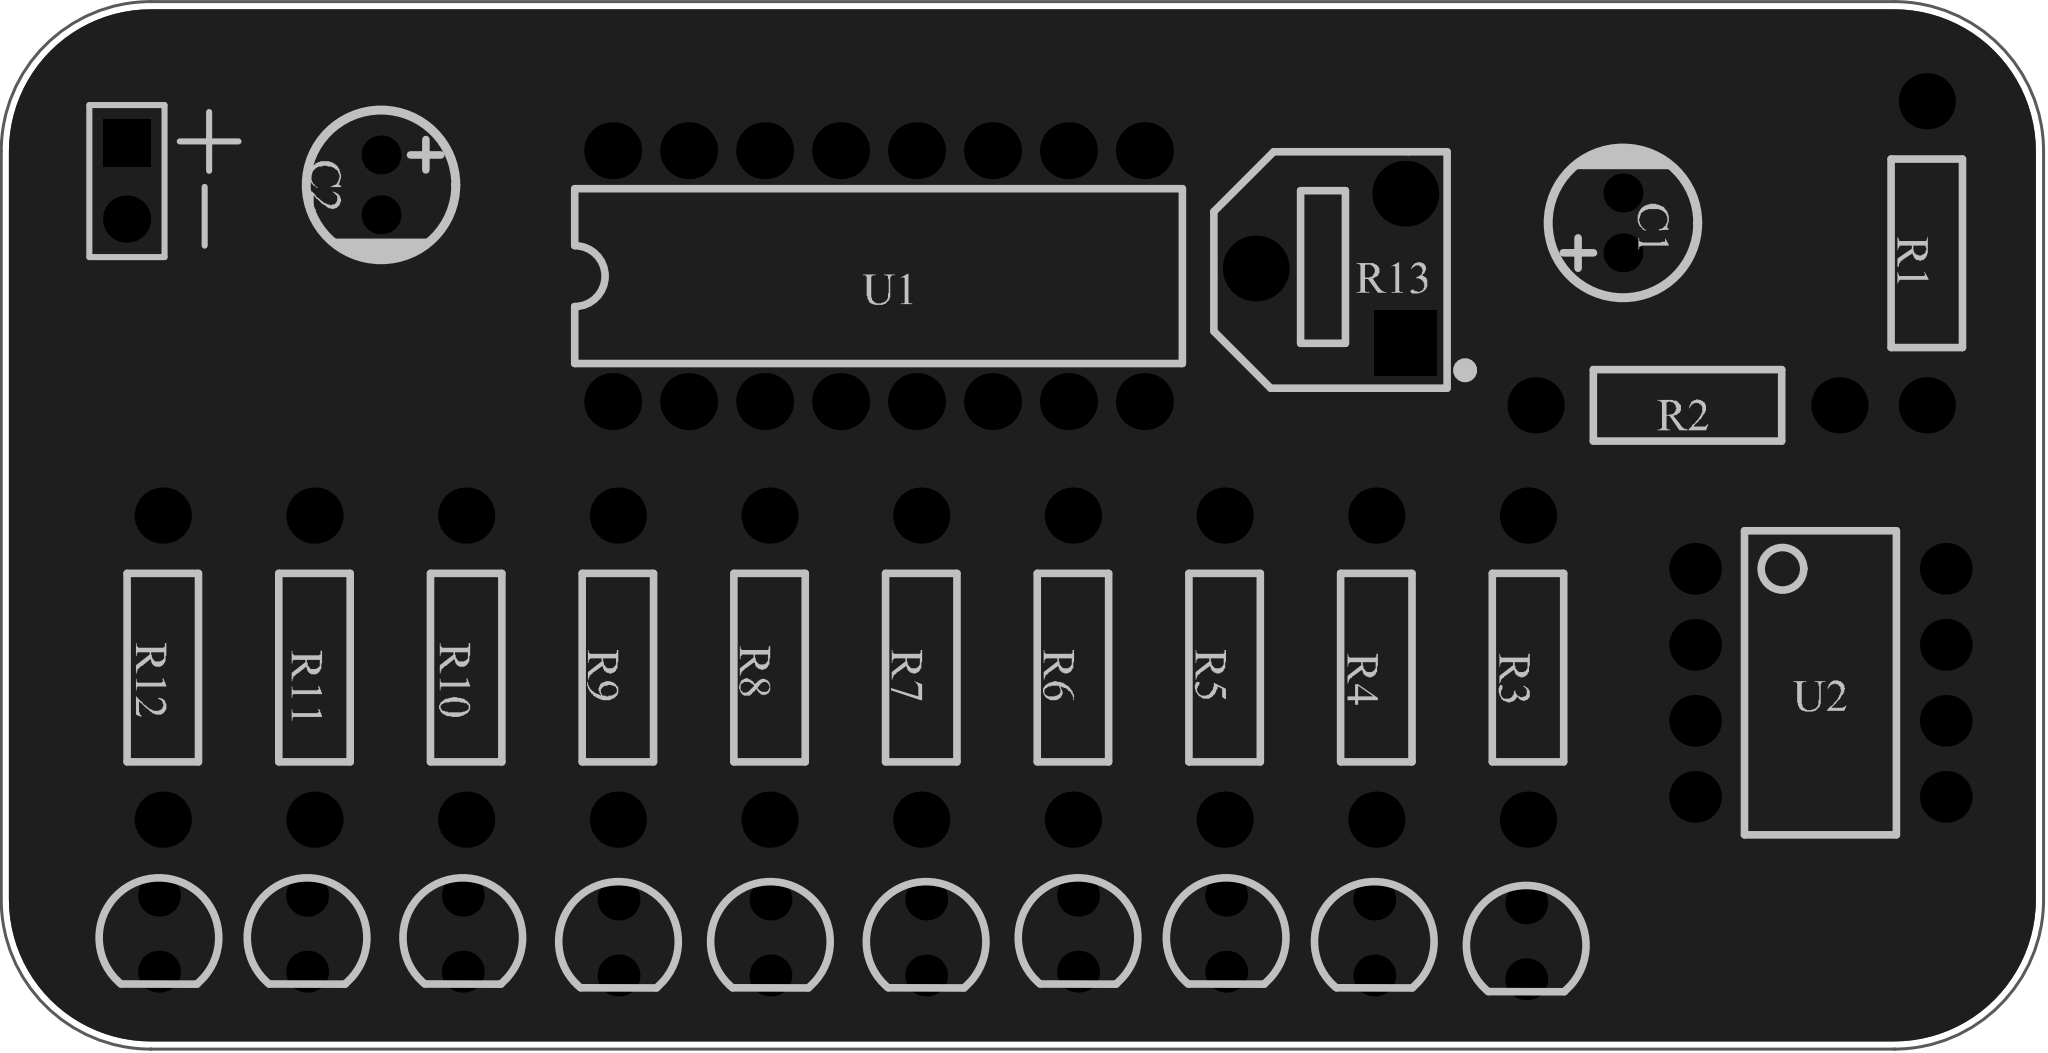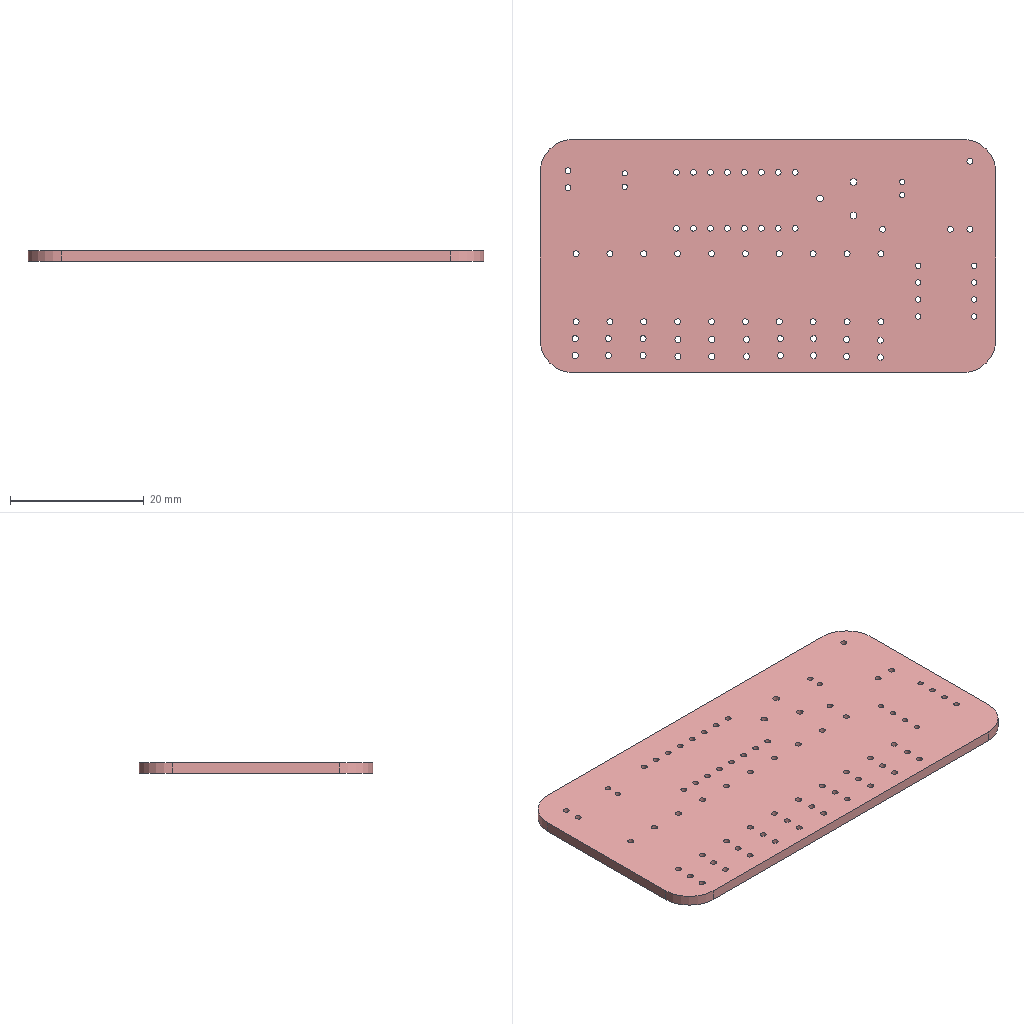Circuit board layout | Altium Designer | box 68.3 x 35 x 1.6 mm
Layer stack:
# Altium Designer layer stack of  (unit mm; dielectric type: 0 none, 1 core, 2 prepreg, 3 surface material)
index,name,kind,layer,copper_thickness_mm,dielectric_type,dielectric_thickness_mm,dielectric_material,dielectric_constant
0,Top Paste Mask Layer,other,,,,,,
1,Top Silkscreen Layer,other,,,,,,
2,Top Solder Mask Layer,dielectric,,,3,0.01,,3.3
3,Top Layer,copper,Top Layer,0.035,,,,
4,Dielectric1,dielectric,,,3,1.51,FR4,4.5
5,Bottom Layer,copper,Bottom Layer,0.035,,,,
6,Bottom Solder Mask Layer,dielectric,,,3,0.01,,3.3
7,Bottom Silkscreen Layer,other,,,,,,
8,Bottom Paste Mask Layer,other,,,,,,
# drill layer pairs: low layer,high layer
drill_pair,Top Layer,Bottom Layer
Part placement:
Designator,Comment,Layer,Footprint,Center-X(mm),Center-Y(mm),Rotation
C1,1uF,TopLayer,CAP-TH_BD5.0-P2.00-D0.8-FD,130.699,104.441,90
C2,1uF,TopLayer,CAP-TH_BD5.0-P2.00-D0.8-FD,89.17,105.711,270
H1,HDR-F-2.54_1x2,TopLayer,HDR-F-2.54_1X2,80.661,105.838,270
LED1,LED-TH-3mm_R,TopLayer,LED-TH_BD3.0_RED,127.466,80.438,0
LED2,LED-TH-3mm_R,TopLayer,LED-TH_BD3.0_RED,122.386,80.565,0
LED3,LED-TH-3mm_R,TopLayer,LED-TH_BD3.0_RED,117.433,80.692,0
LED4,LED-TH-3mm_R,TopLayer,LED-TH_BD3.0_RED,112.48,80.692,0
LED5,LED-TH-3mm_R,TopLayer,LED-TH_BD3.0_RED,107.4,80.565,0
LED6,LED-TH-3mm_R,TopLayer,LED-TH_BD3.0_RED,102.193,80.565,0
LED7,LED-TH-3mm_R,TopLayer,LED-TH_BD3.0_RED,97.113,80.565,0
LED8,LED-TH-3mm_R,TopLayer,LED-TH_BD3.0_RED,91.906,80.692,0
LED9,LED-TH-3mm_R,TopLayer,LED-TH_BD3.0_RED,86.699,80.692,0
LED10,LED-TH-3mm_R,TopLayer,LED-TH_BD3.0_RED,81.746,80.692,0
R2,10k,TopLayer,R_AXIAL-0.4,132.858,98.345,0
R3,1k,TopLayer,R_AXIAL-0.4,127.524,89.582,270
R4,1k,TopLayer,R_AXIAL-0.4,122.452,89.582,270
R5,1k,TopLayer,R_AXIAL-0.4,117.379,89.582,270
R6,1k,TopLayer,R_AXIAL-0.4,112.307,89.582,270
R7,1k,TopLayer,R_AXIAL-0.4,107.234,89.582,270
R8,1k,TopLayer,R_AXIAL-0.4,102.162,89.582,270
R9,1k,TopLayer,R_AXIAL-0.4,97.09,89.582,270
R10,1k,TopLayer,R_AXIAL-0.4,92.017,89.582,270
R11,1k,TopLayer,R_AXIAL-0.4,86.945,89.582,270
R12,1k,TopLayer,R_AXIAL-0.4,81.873,89.582,270
U1,CD4017,TopLayer,CD4017,105.807,102.663,0
U2,NE555,TopLayer,DIP08-KIT,137.303,89.074,270
R1,2.2k,TopLayer,R_AXIAL-0.4,140.859,103.425,90
R13,50K,TopLayer,RES-ADJ-SMD_RM065-V1,120.92,102.917,90
Pad and via stacks:
# Altium Designer via and pad stacks of  (unit mm). Each distinct definition once, with the count of objects using it.
# via: kind,start_layer,end_layer,hole_mm,diameter_mm,mode(0 simple;1 top-mid-bottom;2 full stack),diameter_per_layer,count,example_net
# pad: kind,layer,hole_mm,hole_type(0 round;1 square;2 slot),plating,top_size,top_shape(1 round;2 rect;3 octagon;9 rounded rect),mid_size,bottom_size,mode,footprint,size_per_layer,count,example
pad,Multi-Layer,0.8,0,plated,1.3x1.3,1,1.3x1.3,1.3x1.3,0,CAP-TH_BD5.0-P2.00-D0.8-FD,,4,C1.1
pad,Multi-Layer,0.889,0,plated,1.575x1.575,2,1.575x1.575,1.575x1.575,0,HDR-F-2.54_1X2,,1,H1.1
pad,Multi-Layer,0.889,0,plated,1.575x1.575,1,1.575x1.575,1.575x1.575,0,HDR-F-2.54_1X2,,1,H1.2
pad,Multi-Layer,0.9,0,plated,1.4x1.4,1,1.4x1.4,1.4x1.4,0,LED-TH_BD3.0_RED,,20,LED1.1
pad,Multi-Layer,0.8992,0,plated,1.88x1.88,1,1.88x1.88,1.88x1.88,0,R_AXIAL-0.4,,24,R2.1
pad,Multi-Layer,0.8636,0,plated,1.905x1.905,1,1.905x1.905,1.905x1.905,0,CD4017,,16,U1.1
pad,Multi-Layer,0.8128,0,plated,1.727x1.727,1,1.727x1.727,1.727x1.727,0,DIP08-KIT,,8,U2.1
pad,Multi-Layer,1,0,plated,2.2x2.1,2,2.2x2.1,2.2x2.1,0,RES-ADJ-SMD_RM065-V1,,1,R13.1
pad,Multi-Layer,1,0,plated,2.2x2.2,1,2.2x2.2,2.2x2.2,0,RES-ADJ-SMD_RM065-V1,,2,R13.3
Copper pours:
name,layer,net,type(0 solid;1 hatched;2 none)
Bottom Layer-GND,Bottom Layer,GND,0
Top Layer-GND,Top Layer,GND,0
Design rules, without the lines most boards share:
# Altium Designer design rules of  (exported by Altium Designer, unit mm)
# columns: name | kind | enabled | priority | scope1 | scope2 | descriptor | typed fields (field=value)
GND | 0 | enabled | 1 | (InNet('GND')) | All | Clearance Constraint (Gap=5.984mil) ((InNet('GND'))),(All) | gap=0.152
GND_1 | 63 | enabled | 1 | All | All | Board Clearance Constraint (Gap=0mil) (All) |
VCC | 0 | enabled | 2 | (InNet('VCC')) | All | Clearance Constraint (Gap=5.984mil) ((InNet('VCC'))),(All) | gap=0.152
VCC_1 | 63 | enabled | 2 | All | All | Board Clearance Constraint (Gap=0mil) (All) |
Plane_Default | 0 | disabled | 3 | All | All | Clearance Constraint (Gap=5.984mil) (Disabled)(All),(All) | gap=0.152
Plane_Default_1 | 63 | disabled | 3 | All | All | Board Clearance Constraint (Gap=0mil) (Disabled)(All) |
Plane_GND | 0 | disabled | 4 | All | All | Clearance Constraint (Gap=5.984mil) (Disabled)(All),(All) | gap=0.152
Plane_GND_1 | 63 | disabled | 4 | All | All | Board Clearance Constraint (Gap=0mil) (Disabled)(All) |
Plane_VCC | 0 | disabled | 5 | All | All | Clearance Constraint (Gap=5.984mil) (Disabled)(All),(All) | gap=0.152
Plane_VCC_1 | 63 | disabled | 5 | All | All | Board Clearance Constraint (Gap=0mil) (Disabled)(All) |
Copper_gge7237 | 0 | disabled | 6 | All | All | Clearance Constraint (Gap=5.984mil) (Disabled)(All),(All) | gap=0.152
Copper_gge7237_1 | 63 | disabled | 6 | All | All | Board Clearance Constraint (Gap=0mil) (Disabled)(All) |
Copper_gge7231 | 0 | disabled | 7 | All | All | Clearance Constraint (Gap=5.984mil) (Disabled)(All),(All) | gap=0.152
Copper_gge7231_1 | 63 | disabled | 7 | All | All | Board Clearance Constraint (Gap=0mil) (Disabled)(All) |
Default | 0 | enabled | 8 | All | All | Clearance Constraint (Gap=5.984mil) (All),(All) | gap=0.152
Default_1 | 63 | enabled | 8 | All | All | Board Clearance Constraint (Gap=0mil) (All) |
otherClearance | 52 | enabled | 1 | All | All | Hole To Hole Clearance (Gap=11.8mil) (All),(All) | gap=0.2997
GND_2 | 2 | enabled | 1 | (InNet('GND')) | All | Width Constraint (Min=39.4mil) (Max=1000mil) (Preferred=39.4mil) ((InNet('GND'))) |
VCC_2 | 2 | enabled | 2 | (InNet('VCC')) | All | Width Constraint (Min=31.5mil) (Max=1000mil) (Preferred=31.5mil) ((InNet('VCC'))) |
Default_2 | 2 | enabled | 3 | All | All | Width Constraint (Min=19.7mil) (Max=1000mil) (Preferred=19.7mil) (All) |
GND_3 | 11 | enabled | 1 | (InNet('GND')) | All | Routing Via (MinHoleWidth=12.008mil) (MaxHoleWidth=2362mil) (PreferredHoleWidth=12.008mil) (MinWidth=24.016mil) (MaxWidth=3938mil) (PreferedWidth=24.016mil) ((InNet('GND'))) | via_min_hole=0.305 via_max_hole=59.995 via_preferred_diameter=0.61 via_preferred_hole=0.305
VCC_3 | 11 | enabled | 2 | (InNet('VCC')) | All | Routing Via (MinHoleWidth=12.008mil) (MaxHoleWidth=2362mil) (PreferredHoleWidth=12.008mil) (MinWidth=24.016mil) (MaxWidth=3938mil) (PreferedWidth=24.016mil) ((InNet('VCC'))) | via_min_hole=0.305 via_max_hole=59.995 via_preferred_diameter=0.61 via_preferred_hole=0.305
Default_3 | 11 | enabled | 3 | All | All | Routing Via (MinHoleWidth=12.008mil) (MaxHoleWidth=2362mil) (PreferredHoleWidth=12.008mil) (MinWidth=24.016mil) (MaxWidth=3938mil) (PreferedWidth=24.016mil) (All) | via_min_hole=0.305 via_max_hole=59.995 via_preferred_diameter=0.61 via_preferred_hole=0.305
GND_4 | 6 | disabled | 1 | All | All | Power Plane Connect Rule(Relief Connect )(Expansion=20mil) (Conductor Width=0mil) (Air Gap=10mil) (Entries=4) (Disabled)(All) | relief_conductor_width=0 relief_entries=4 relief_expansion=0.508
VCC_4 | 6 | disabled | 2 | All | All | Power Plane Connect Rule(Relief Connect )(Expansion=20mil) (Conductor Width=0mil) (Air Gap=10mil) (Entries=4) (Disabled)(All) | relief_conductor_width=0 relief_entries=4 relief_expansion=0.508
Default_4 | 6 | enabled | 3 | All | All | Power Plane Connect Rule(Relief Connect )(Expansion=20mil) (Conductor Width=0mil) (Air Gap=10mil) (Entries=4) (All) | relief_conductor_width=0 relief_entries=4 relief_expansion=0.508
gge7231 | 20 | disabled | 1 | All | All | Polygon Connect Rule(Relief Connect )(Conductor Width=0mil) (Relief Angle=90 Angle) (Entries=4) (Air Gap Width=10mil) (Disabled)(All),(All) | connect_style(0=relief,1=direct,2=none)=0 relief_conductor_width=0 relief_entries=4
gge7237 | 20 | enabled | 2 | All | All | Polygon Connect Rule(Relief Connect )(Conductor Width=0mil) (Relief Angle=90 Angle) (Entries=4) (Air Gap Width=10mil) (All),(All) | connect_style(0=relief,1=direct,2=none)=0 relief_conductor_width=0 relief_entries=4
Common | 14 | enabled | 1 | All | All | Paste Mask Expansion (Expansion =0mil) (All) | expansion=0
Common_1 | 13 | enabled | 1 | All | All | Solder Mask Expansion (Expansion =0mil) (All) | expansion=0